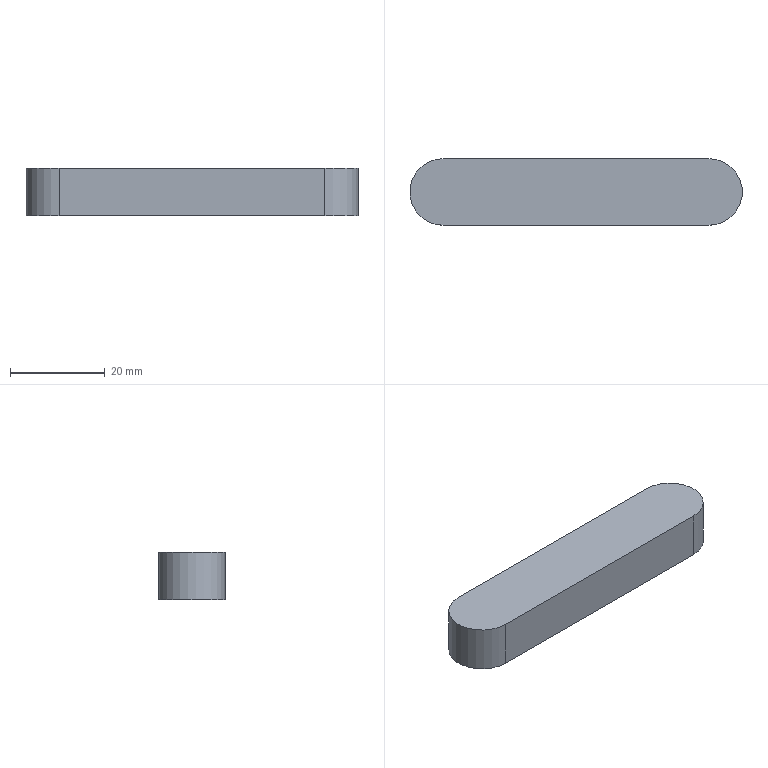Part | NX | 1 solid | 6 faces | box 70 x 14 x 10 mm | volume 9379 mm3 | plane 4 | cylinder 2 | commonest cylinder face diameters 14 x2
STEP:
#1=CARTESIAN_POINT('',(-28.,-7.,10.));
#2=VERTEX_POINT('',#1);
#3=CARTESIAN_POINT('',(28.,-7.,10.));
#4=VERTEX_POINT('',#3);
#5=CARTESIAN_POINT('',(-35.,-7.,10.));
#6=DIRECTION('',(1.,0.,0.));
#7=VECTOR('',#6,1.);
#8=LINE('',#5,#7);
#9=EDGE_CURVE('',#2,#4,#8,.T.);
#10=ORIENTED_EDGE('',*,*,#9,.F.);
#11=CARTESIAN_POINT('',(-28.,-7.,0.));
#12=VERTEX_POINT('',#11);
#13=CARTESIAN_POINT('',(-28.,-7.,10.));
#14=DIRECTION('',(0.,0.,-1.));
#15=VECTOR('',#14,1.);
#16=LINE('',#13,#15);
#17=EDGE_CURVE('',#2,#12,#16,.T.);
#18=ORIENTED_EDGE('',*,*,#17,.T.);
#19=CARTESIAN_POINT('',(28.,-7.,0.));
#20=VERTEX_POINT('',#19);
#21=CARTESIAN_POINT('',(-35.,-7.,0.));
#22=DIRECTION('',(1.,0.,0.));
#23=VECTOR('',#22,1.);
#24=LINE('',#21,#23);
#25=EDGE_CURVE('',#12,#20,#24,.T.);
#26=ORIENTED_EDGE('',*,*,#25,.T.);
#27=CARTESIAN_POINT('',(28.,-7.,10.));
#28=DIRECTION('',(0.,0.,1.));
#29=VECTOR('',#28,1.);
#30=LINE('',#27,#29);
#31=EDGE_CURVE('',#20,#4,#30,.T.);
#32=ORIENTED_EDGE('',*,*,#31,.T.);
#33=EDGE_LOOP('',(#10,#18,#26,#32));
#34=FACE_OUTER_BOUND('',#33,.T.);
#35=CARTESIAN_POINT('',(-35.,-7.,10.));
#36=DIRECTION('',(0.,1.,0.));
#37=DIRECTION('',(0.,0.,-1.));
#38=AXIS2_PLACEMENT_3D('',#35,#36,#37);
#39=PLANE('',#38);
#40=ADVANCED_FACE('',(#34),#39,.F.);
#41=CARTESIAN_POINT('',(28.,7.,0.));
#42=VERTEX_POINT('',#41);
#43=CARTESIAN_POINT('',(-28.,7.,0.));
#44=VERTEX_POINT('',#43);
#45=CARTESIAN_POINT('',(35.,7.,0.));
#46=DIRECTION('',(-1.,0.,0.));
#47=VECTOR('',#46,1.);
#48=LINE('',#45,#47);
#49=EDGE_CURVE('',#42,#44,#48,.T.);
#50=ORIENTED_EDGE('',*,*,#49,.T.);
#51=CARTESIAN_POINT('',(-28.,7.,10.));
#52=VERTEX_POINT('',#51);
#53=CARTESIAN_POINT('',(-28.,7.,10.));
#54=DIRECTION('',(0.,0.,1.));
#55=VECTOR('',#54,1.);
#56=LINE('',#53,#55);
#57=EDGE_CURVE('',#44,#52,#56,.T.);
#58=ORIENTED_EDGE('',*,*,#57,.T.);
#59=CARTESIAN_POINT('',(28.,7.,10.));
#60=VERTEX_POINT('',#59);
#61=CARTESIAN_POINT('',(35.,7.,10.));
#62=DIRECTION('',(-1.,0.,0.));
#63=VECTOR('',#62,1.);
#64=LINE('',#61,#63);
#65=EDGE_CURVE('',#60,#52,#64,.T.);
#66=ORIENTED_EDGE('',*,*,#65,.F.);
#67=CARTESIAN_POINT('',(28.,7.,10.));
#68=DIRECTION('',(0.,0.,-1.));
#69=VECTOR('',#68,1.);
#70=LINE('',#67,#69);
#71=EDGE_CURVE('',#60,#42,#70,.T.);
#72=ORIENTED_EDGE('',*,*,#71,.T.);
#73=EDGE_LOOP('',(#50,#58,#66,#72));
#74=FACE_OUTER_BOUND('',#73,.T.);
#75=CARTESIAN_POINT('',(35.,7.,10.));
#76=DIRECTION('',(0.,-1.,0.));
#77=DIRECTION('',(0.,0.,1.));
#78=AXIS2_PLACEMENT_3D('',#75,#76,#77);
#79=PLANE('',#78);
#80=ADVANCED_FACE('',(#74),#79,.F.);
#81=ORIENTED_EDGE('',*,*,#65,.T.);
#82=CARTESIAN_POINT('',(-28.,0.,10.));
#83=DIRECTION('',(0.,0.,1.));
#84=DIRECTION('',(1.,0.,0.));
#85=AXIS2_PLACEMENT_3D('',#82,#83,#84);
#86=CIRCLE('',#85,7.);
#87=EDGE_CURVE('',#52,#2,#86,.T.);
#88=ORIENTED_EDGE('',*,*,#87,.T.);
#89=ORIENTED_EDGE('',*,*,#9,.T.);
#90=CARTESIAN_POINT('',(28.,0.,10.));
#91=DIRECTION('',(0.,0.,1.));
#92=DIRECTION('',(1.,0.,0.));
#93=AXIS2_PLACEMENT_3D('',#90,#91,#92);
#94=CIRCLE('',#93,7.);
#95=EDGE_CURVE('',#4,#60,#94,.T.);
#96=ORIENTED_EDGE('',*,*,#95,.T.);
#97=EDGE_LOOP('',(#81,#88,#89,#96));
#98=FACE_OUTER_BOUND('',#97,.T.);
#99=CARTESIAN_POINT('',(0.,0.,10.));
#100=DIRECTION('',(0.,0.,1.));
#101=DIRECTION('',(-1.,0.,0.));
#102=AXIS2_PLACEMENT_3D('',#99,#100,#101);
#103=PLANE('',#102);
#104=ADVANCED_FACE('',(#98),#103,.T.);
#105=CARTESIAN_POINT('',(-28.,0.,0.));
#106=DIRECTION('',(0.,0.,-1.));
#107=DIRECTION('',(1.,0.,0.));
#108=AXIS2_PLACEMENT_3D('',#105,#106,#107);
#109=CIRCLE('',#108,7.);
#110=EDGE_CURVE('',#12,#44,#109,.T.);
#111=ORIENTED_EDGE('',*,*,#110,.T.);
#112=ORIENTED_EDGE('',*,*,#49,.F.);
#113=CARTESIAN_POINT('',(28.,0.,0.));
#114=DIRECTION('',(0.,0.,-1.));
#115=DIRECTION('',(1.,0.,0.));
#116=AXIS2_PLACEMENT_3D('',#113,#114,#115);
#117=CIRCLE('',#116,7.);
#118=EDGE_CURVE('',#42,#20,#117,.T.);
#119=ORIENTED_EDGE('',*,*,#118,.T.);
#120=ORIENTED_EDGE('',*,*,#25,.F.);
#121=EDGE_LOOP('',(#111,#112,#119,#120));
#122=FACE_OUTER_BOUND('',#121,.T.);
#123=CARTESIAN_POINT('',(0.,0.,0.));
#124=DIRECTION('',(0.,0.,1.));
#125=DIRECTION('',(-1.,0.,0.));
#126=AXIS2_PLACEMENT_3D('',#123,#124,#125);
#127=PLANE('',#126);
#128=ADVANCED_FACE('',(#122),#127,.F.);
#129=ORIENTED_EDGE('',*,*,#17,.F.);
#130=ORIENTED_EDGE('',*,*,#87,.F.);
#131=ORIENTED_EDGE('',*,*,#57,.F.);
#132=ORIENTED_EDGE('',*,*,#110,.F.);
#133=EDGE_LOOP('',(#129,#130,#131,#132));
#134=FACE_OUTER_BOUND('',#133,.T.);
#135=CARTESIAN_POINT('',(-28.,0.,10.));
#136=DIRECTION('',(0.,0.,-1.));
#137=DIRECTION('',(1.,0.,0.));
#138=AXIS2_PLACEMENT_3D('',#135,#136,#137);
#139=CYLINDRICAL_SURFACE('',#138,7.);
#140=ADVANCED_FACE('',(#134),#139,.T.);
#141=ORIENTED_EDGE('',*,*,#71,.F.);
#142=ORIENTED_EDGE('',*,*,#95,.F.);
#143=ORIENTED_EDGE('',*,*,#31,.F.);
#144=ORIENTED_EDGE('',*,*,#118,.F.);
#145=EDGE_LOOP('',(#141,#142,#143,#144));
#146=FACE_OUTER_BOUND('',#145,.T.);
#147=CARTESIAN_POINT('',(28.,0.,10.));
#148=DIRECTION('',(0.,0.,-1.));
#149=DIRECTION('',(1.,0.,0.));
#150=AXIS2_PLACEMENT_3D('',#147,#148,#149);
#151=CYLINDRICAL_SURFACE('',#150,7.);
#152=ADVANCED_FACE('',(#146),#151,.T.);
#153=CLOSED_SHELL('',(#40,#80,#104,#128,#140,#152));
#154=MANIFOLD_SOLID_BREP('',#153);
#155=(LENGTH_UNIT()NAMED_UNIT(*)SI_UNIT(.MILLI.,.METRE.));
#156=UNCERTAINTY_MEASURE_WITH_UNIT(LENGTH_MEASURE(0.00002),#155,'','');
#157=(NAMED_UNIT(*)PLANE_ANGLE_UNIT()SI_UNIT($,.RADIAN.));
#158=PLANE_ANGLE_MEASURE_WITH_UNIT(PLANE_ANGLE_MEASURE(0.01745),#157);
#159=DIMENSIONAL_EXPONENTS(0.,0.,0.,0.,0.,0.,0.);
#160=(CONVERSION_BASED_UNIT('DEGREE',#158)NAMED_UNIT(#159)PLANE_ANGLE_UNIT());
#161=(NAMED_UNIT(*)SI_UNIT($,.STERADIAN.)SOLID_ANGLE_UNIT());
#162=(GEOMETRIC_REPRESENTATION_CONTEXT(3)GLOBAL_UNCERTAINTY_ASSIGNED_CONTEXT((#156))GLOBAL_UNIT_ASSIGNED_CONTEXT((#155,#160,#161))REPRESENTATION_CONTEXT('',''));
#163=ADVANCED_BREP_SHAPE_REPRESENTATION('',(#154),#162);